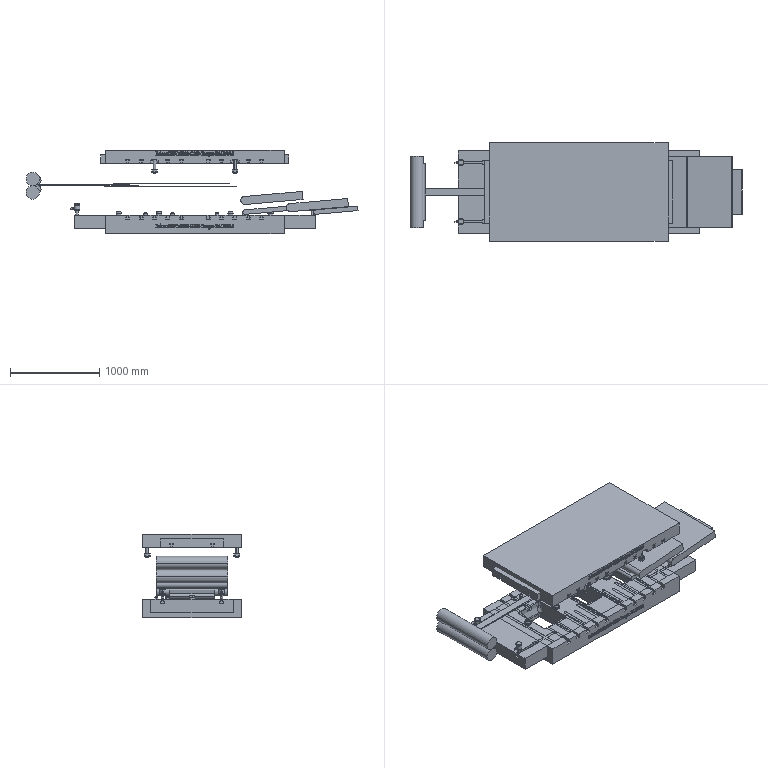Part | CATIA | 35 solids | 7642 faces | volume 1311212838 mm3 | plane 2598 | spline 1691 | other 1540 | cylinder 1232 | cone 264 | sphere 248 | torus 69 | commonest cylinder face diameters 66 x424 46 x93 28 x73 21 x64 2 x60 5 x52